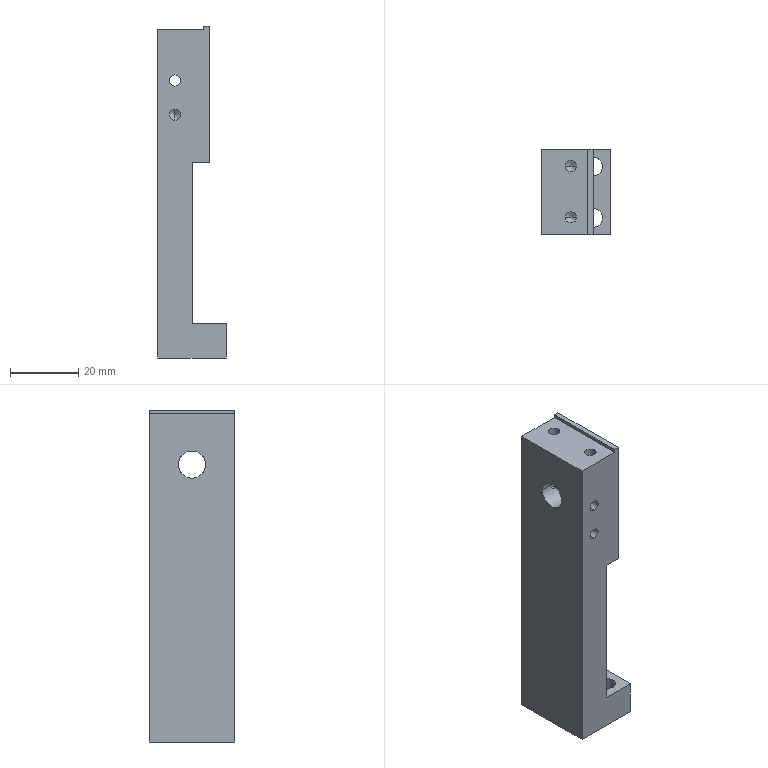Part | STEP file | 11-FG-B02911 | 1 solid | 38 faces | box 20 x 25 x 97.4 mm | volume 29767 mm3 | cylinder 18 | plane 12 | cone 8 | commonest cylinder face diameters 3.3 x12 5.5 x4 8 x2
STEP:
#1=CARTESIAN_POINT('',(5.,14.9,69.75));
#2=VERTEX_POINT('',#1);
#3=CARTESIAN_POINT('',(5.,14.9,73.05));
#4=VERTEX_POINT('',#3);
#5=CARTESIAN_POINT('',(5.,14.9,71.4));
#6=DIRECTION('',(0.,1.,0.));
#7=DIRECTION('',(0.,0.,1.));
#8=AXIS2_PLACEMENT_3D('',#5,#6,#7);
#9=CIRCLE('',#8,1.65);
#10=EDGE_CURVE('',#2,#4,#9,.T.);
#11=ORIENTED_EDGE('',*,*,#10,.F.);
#12=CARTESIAN_POINT('',(5.,25.,69.75));
#13=VERTEX_POINT('',#12);
#14=CARTESIAN_POINT('',(5.,25.,69.75));
#15=DIRECTION('',(0.,1.,0.));
#16=VECTOR('',#15,1000.);
#17=LINE('',#14,#16);
#18=EDGE_CURVE('',#2,#13,#17,.T.);
#19=ORIENTED_EDGE('',*,*,#18,.T.);
#20=CARTESIAN_POINT('',(5.,25.,73.05));
#21=VERTEX_POINT('',#20);
#22=CARTESIAN_POINT('',(5.,25.,71.4));
#23=DIRECTION('',(0.,1.,0.));
#24=DIRECTION('',(0.,0.,1.));
#25=AXIS2_PLACEMENT_3D('',#22,#23,#24);
#26=CIRCLE('',#25,1.65);
#27=EDGE_CURVE('',#13,#21,#26,.T.);
#28=ORIENTED_EDGE('',*,*,#27,.T.);
#29=CARTESIAN_POINT('',(5.,25.,73.05));
#30=DIRECTION('',(0.,1.,0.));
#31=VECTOR('',#30,1000.);
#32=LINE('',#29,#31);
#33=EDGE_CURVE('',#4,#21,#32,.T.);
#34=ORIENTED_EDGE('',*,*,#33,.F.);
#35=EDGE_LOOP('',(#11,#19,#28,#34));
#36=FACE_OUTER_BOUND('',#35,.T.);
#37=CARTESIAN_POINT('',(5.,25.,71.4));
#38=DIRECTION('',(0.,1.,0.));
#39=DIRECTION('',(0.,0.,1.));
#40=AXIS2_PLACEMENT_3D('',#37,#38,#39);
#41=CYLINDRICAL_SURFACE('',#40,1.65);
#42=ADVANCED_FACE('',(#36),#41,.F.);
#43=CARTESIAN_POINT('',(5.,13.909,71.4));
#44=VERTEX_POINT('',#43);
#45=CARTESIAN_POINT('',(5.,14.9,73.05));
#46=DIRECTION('',(0.,0.515,0.8572));
#47=VECTOR('',#46,1000.);
#48=LINE('',#45,#47);
#49=EDGE_CURVE('',#44,#4,#48,.T.);
#50=ORIENTED_EDGE('',*,*,#49,.F.);
#51=CARTESIAN_POINT('',(5.,14.9,69.75));
#52=DIRECTION('',(0.,0.515,-0.8572));
#53=VECTOR('',#52,1000.);
#54=LINE('',#51,#53);
#55=EDGE_CURVE('',#44,#2,#54,.T.);
#56=ORIENTED_EDGE('',*,*,#55,.T.);
#57=ORIENTED_EDGE('',*,*,#10,.T.);
#58=EDGE_LOOP('',(#50,#56,#57));
#59=FACE_OUTER_BOUND('',#58,.T.);
#60=CARTESIAN_POINT('',(5.,14.9,71.4));
#61=DIRECTION('',(0.,1.,0.));
#62=DIRECTION('',(0.,0.,1.));
#63=AXIS2_PLACEMENT_3D('',#60,#61,#62);
#64=CONICAL_SURFACE('',#63,1.65,1.03);
#65=ADVANCED_FACE('',(#59),#64,.F.);
#66=CARTESIAN_POINT('',(5.,10.1,73.05));
#67=VERTEX_POINT('',#66);
#68=CARTESIAN_POINT('',(5.,10.1,69.75));
#69=VERTEX_POINT('',#68);
#70=CARTESIAN_POINT('',(5.,10.1,71.4));
#71=DIRECTION('',(0.,-1.,0.));
#72=DIRECTION('',(0.,0.,-1.));
#73=AXIS2_PLACEMENT_3D('',#70,#71,#72);
#74=CIRCLE('',#73,1.65);
#75=EDGE_CURVE('',#67,#69,#74,.T.);
#76=ORIENTED_EDGE('',*,*,#75,.F.);
#77=CARTESIAN_POINT('',(5.,0.,73.05));
#78=VERTEX_POINT('',#77);
#79=CARTESIAN_POINT('',(5.,0.,73.05));
#80=DIRECTION('',(0.,-1.,0.));
#81=VECTOR('',#80,1000.);
#82=LINE('',#79,#81);
#83=EDGE_CURVE('',#67,#78,#82,.T.);
#84=ORIENTED_EDGE('',*,*,#83,.T.);
#85=CARTESIAN_POINT('',(5.,0.,69.75));
#86=VERTEX_POINT('',#85);
#87=CARTESIAN_POINT('',(5.,0.,71.4));
#88=DIRECTION('',(0.,-1.,0.));
#89=DIRECTION('',(0.,0.,-1.));
#90=AXIS2_PLACEMENT_3D('',#87,#88,#89);
#91=CIRCLE('',#90,1.65);
#92=EDGE_CURVE('',#78,#86,#91,.T.);
#93=ORIENTED_EDGE('',*,*,#92,.T.);
#94=CARTESIAN_POINT('',(5.,0.,69.75));
#95=DIRECTION('',(0.,-1.,0.));
#96=VECTOR('',#95,1000.);
#97=LINE('',#94,#96);
#98=EDGE_CURVE('',#69,#86,#97,.T.);
#99=ORIENTED_EDGE('',*,*,#98,.F.);
#100=EDGE_LOOP('',(#76,#84,#93,#99));
#101=FACE_OUTER_BOUND('',#100,.T.);
#102=CARTESIAN_POINT('',(5.,0.,71.4));
#103=DIRECTION('',(0.,-1.,0.));
#104=DIRECTION('',(0.,0.,-1.));
#105=AXIS2_PLACEMENT_3D('',#102,#103,#104);
#106=CYLINDRICAL_SURFACE('',#105,1.65);
#107=ADVANCED_FACE('',(#101),#106,.F.);
#108=CARTESIAN_POINT('',(5.,11.091,71.4));
#109=VERTEX_POINT('',#108);
#110=CARTESIAN_POINT('',(5.,10.1,69.75));
#111=DIRECTION('',(0.,-0.515,-0.8572));
#112=VECTOR('',#111,1000.);
#113=LINE('',#110,#112);
#114=EDGE_CURVE('',#109,#69,#113,.T.);
#115=ORIENTED_EDGE('',*,*,#114,.F.);
#116=CARTESIAN_POINT('',(5.,10.1,73.05));
#117=DIRECTION('',(0.,-0.515,0.8572));
#118=VECTOR('',#117,1000.);
#119=LINE('',#116,#118);
#120=EDGE_CURVE('',#109,#67,#119,.T.);
#121=ORIENTED_EDGE('',*,*,#120,.T.);
#122=ORIENTED_EDGE('',*,*,#75,.T.);
#123=EDGE_LOOP('',(#115,#121,#122));
#124=FACE_OUTER_BOUND('',#123,.T.);
#125=CARTESIAN_POINT('',(5.,10.1,71.4));
#126=DIRECTION('',(0.,-1.,0.));
#127=DIRECTION('',(0.,0.,-1.));
#128=AXIS2_PLACEMENT_3D('',#125,#126,#127);
#129=CONICAL_SURFACE('',#128,1.65,1.03);
#130=ADVANCED_FACE('',(#124),#129,.F.);
#131=CARTESIAN_POINT('',(5.,16.144,79.75));
#132=VERTEX_POINT('',#131);
#133=CARTESIAN_POINT('',(3.35,16.5,81.4));
#134=VERTEX_POINT('',#133);
#135=CARTESIAN_POINT('',(5.,16.144,79.75));
#136=CARTESIAN_POINT('',(4.891,16.144,79.75));
#137=CARTESIAN_POINT('',(4.781,16.149,79.761));
#138=CARTESIAN_POINT('',(4.568,16.168,79.804));
#139=CARTESIAN_POINT('',(4.464,16.182,79.836));
#140=CARTESIAN_POINT('',(4.165,16.233,79.961));
#141=CARTESIAN_POINT('',(3.985,16.28,80.082));
#142=CARTESIAN_POINT('',(3.757,16.349,80.31));
#143=CARTESIAN_POINT('',(3.689,16.372,80.392));
#144=CARTESIAN_POINT('',(3.571,16.414,80.569));
#145=CARTESIAN_POINT('',(3.519,16.433,80.665));
#146=CARTESIAN_POINT('',(3.436,16.465,80.865));
#147=CARTESIAN_POINT('',(3.404,16.478,80.968));
#148=CARTESIAN_POINT('',(3.361,16.495,81.181));
#149=CARTESIAN_POINT('',(3.35,16.5,81.291));
#150=CARTESIAN_POINT('',(3.35,16.5,81.4));
#151=B_SPLINE_CURVE_WITH_KNOTS('',3,(#135,#136,#137,#138,#139,#140,#141,#142,#143,#144,#145,#146,#147,#148,#149,#150),.UNSPECIFIED.,.F.,.F.,(4,2,2,2,2,2,2,4),(0.005217,0.005543,0.005869,0.006521,0.006847,0.007172,0.007498,0.007824),.UNSPECIFIED.);
#152=EDGE_CURVE('',#132,#134,#151,.T.);
#153=ORIENTED_EDGE('',*,*,#152,.F.);
#154=CARTESIAN_POINT('',(5.,25.,79.75));
#155=VERTEX_POINT('',#154);
#156=CARTESIAN_POINT('',(5.,25.,79.75));
#157=DIRECTION('',(0.,1.,0.));
#158=VECTOR('',#157,1000.);
#159=LINE('',#156,#158);
#160=EDGE_CURVE('',#132,#155,#159,.T.);
#161=ORIENTED_EDGE('',*,*,#160,.T.);
#162=CARTESIAN_POINT('',(5.,25.,83.05));
#163=VERTEX_POINT('',#162);
#164=CARTESIAN_POINT('',(5.,25.,81.4));
#165=DIRECTION('',(0.,1.,0.));
#166=DIRECTION('',(0.,0.,1.));
#167=AXIS2_PLACEMENT_3D('',#164,#165,#166);
#168=CIRCLE('',#167,1.65);
#169=EDGE_CURVE('',#155,#163,#168,.T.);
#170=ORIENTED_EDGE('',*,*,#169,.T.);
#171=CARTESIAN_POINT('',(5.,16.144,83.05));
#172=VERTEX_POINT('',#171);
#173=CARTESIAN_POINT('',(5.,25.,83.05));
#174=DIRECTION('',(0.,1.,0.));
#175=VECTOR('',#174,1000.);
#176=LINE('',#173,#175);
#177=EDGE_CURVE('',#172,#163,#176,.T.);
#178=ORIENTED_EDGE('',*,*,#177,.F.);
#179=CARTESIAN_POINT('',(3.35,16.5,81.4));
#180=CARTESIAN_POINT('',(3.35,16.5,81.618));
#181=CARTESIAN_POINT('',(3.394,16.481,81.837));
#182=CARTESIAN_POINT('',(3.519,16.433,82.135));
#183=CARTESIAN_POINT('',(3.571,16.414,82.231));
#184=CARTESIAN_POINT('',(3.69,16.372,82.409));
#185=CARTESIAN_POINT('',(3.758,16.349,82.491));
#186=CARTESIAN_POINT('',(3.909,16.303,82.643));
#187=CARTESIAN_POINT('',(3.993,16.279,82.711));
#188=CARTESIAN_POINT('',(4.17,16.236,82.83));
#189=CARTESIAN_POINT('',(4.264,16.216,82.881));
#190=CARTESIAN_POINT('',(4.565,16.164,83.007));
#191=CARTESIAN_POINT('',(4.779,16.144,83.05));
#192=CARTESIAN_POINT('',(5.,16.144,83.05));
#193=B_SPLINE_CURVE_WITH_KNOTS('',3,(#179,#180,#181,#182,#183,#184,#185,#186,#187,#188,#189,#190,#191,#192),.UNSPECIFIED.,.F.,.F.,(4,2,2,2,2,2,4),(0.007824,0.008476,0.008802,0.009127,0.009453,0.009779,0.01043),.UNSPECIFIED.);
#194=EDGE_CURVE('',#134,#172,#193,.T.);
#195=ORIENTED_EDGE('',*,*,#194,.F.);
#196=EDGE_LOOP('',(#153,#161,#170,#178,#195));
#197=FACE_OUTER_BOUND('',#196,.T.);
#198=CARTESIAN_POINT('',(5.,25.,81.4));
#199=DIRECTION('',(0.,1.,0.));
#200=DIRECTION('',(0.,0.,1.));
#201=AXIS2_PLACEMENT_3D('',#198,#199,#200);
#202=CYLINDRICAL_SURFACE('',#201,1.65);
#203=ADVANCED_FACE('',(#197),#202,.F.);
#204=CARTESIAN_POINT('',(12.25,5.,0.));
#205=VERTEX_POINT('',#204);
#206=CARTESIAN_POINT('',(17.75,5.,0.));
#207=VERTEX_POINT('',#206);
#208=CARTESIAN_POINT('',(15.,5.,0.));
#209=DIRECTION('',(0.,0.,1.));
#210=DIRECTION('',(1.,0.,0.));
#211=AXIS2_PLACEMENT_3D('',#208,#209,#210);
#212=CIRCLE('',#211,2.75);
#213=EDGE_CURVE('',#205,#207,#212,.T.);
#214=ORIENTED_EDGE('',*,*,#213,.F.);
#215=CARTESIAN_POINT('',(12.25,5.,10.));
#216=VERTEX_POINT('',#215);
#217=CARTESIAN_POINT('',(12.25,5.,0.));
#218=DIRECTION('',(0.,0.,1.));
#219=VECTOR('',#218,1000.);
#220=LINE('',#217,#219);
#221=EDGE_CURVE('',#205,#216,#220,.T.);
#222=ORIENTED_EDGE('',*,*,#221,.T.);
#223=CARTESIAN_POINT('',(17.75,5.,10.));
#224=VERTEX_POINT('',#223);
#225=CARTESIAN_POINT('',(15.,5.,10.));
#226=DIRECTION('',(0.,0.,1.));
#227=DIRECTION('',(1.,0.,0.));
#228=AXIS2_PLACEMENT_3D('',#225,#226,#227);
#229=CIRCLE('',#228,2.75);
#230=EDGE_CURVE('',#216,#224,#229,.T.);
#231=ORIENTED_EDGE('',*,*,#230,.T.);
#232=CARTESIAN_POINT('',(17.75,5.,0.));
#233=DIRECTION('',(0.,0.,1.));
#234=VECTOR('',#233,1000.);
#235=LINE('',#232,#234);
#236=EDGE_CURVE('',#207,#224,#235,.T.);
#237=ORIENTED_EDGE('',*,*,#236,.F.);
#238=EDGE_LOOP('',(#214,#222,#231,#237));
#239=FACE_OUTER_BOUND('',#238,.T.);
#240=CARTESIAN_POINT('',(15.,5.,0.));
#241=DIRECTION('',(0.,0.,1.));
#242=DIRECTION('',(1.,0.,0.));
#243=AXIS2_PLACEMENT_3D('',#240,#241,#242);
#244=CYLINDRICAL_SURFACE('',#243,2.75);
#245=ADVANCED_FACE('',(#239),#244,.F.);
#246=CARTESIAN_POINT('',(12.25,20.,0.));
#247=VERTEX_POINT('',#246);
#248=CARTESIAN_POINT('',(17.75,20.,0.));
#249=VERTEX_POINT('',#248);
#250=CARTESIAN_POINT('',(15.,20.,0.));
#251=DIRECTION('',(0.,0.,1.));
#252=DIRECTION('',(1.,0.,0.));
#253=AXIS2_PLACEMENT_3D('',#250,#251,#252);
#254=CIRCLE('',#253,2.75);
#255=EDGE_CURVE('',#247,#249,#254,.T.);
#256=ORIENTED_EDGE('',*,*,#255,.F.);
#257=CARTESIAN_POINT('',(12.25,20.,10.));
#258=VERTEX_POINT('',#257);
#259=CARTESIAN_POINT('',(12.25,20.,0.));
#260=DIRECTION('',(0.,0.,1.));
#261=VECTOR('',#260,1000.);
#262=LINE('',#259,#261);
#263=EDGE_CURVE('',#247,#258,#262,.T.);
#264=ORIENTED_EDGE('',*,*,#263,.T.);
#265=CARTESIAN_POINT('',(17.75,20.,10.));
#266=VERTEX_POINT('',#265);
#267=CARTESIAN_POINT('',(15.,20.,10.));
#268=DIRECTION('',(0.,0.,1.));
#269=DIRECTION('',(1.,0.,0.));
#270=AXIS2_PLACEMENT_3D('',#267,#268,#269);
#271=CIRCLE('',#270,2.75);
#272=EDGE_CURVE('',#258,#266,#271,.T.);
#273=ORIENTED_EDGE('',*,*,#272,.T.);
#274=CARTESIAN_POINT('',(17.75,20.,0.));
#275=DIRECTION('',(0.,0.,1.));
#276=VECTOR('',#275,1000.);
#277=LINE('',#274,#276);
#278=EDGE_CURVE('',#249,#266,#277,.T.);
#279=ORIENTED_EDGE('',*,*,#278,.F.);
#280=EDGE_LOOP('',(#256,#264,#273,#279));
#281=FACE_OUTER_BOUND('',#280,.T.);
#282=CARTESIAN_POINT('',(15.,20.,0.));
#283=DIRECTION('',(0.,0.,1.));
#284=DIRECTION('',(1.,0.,0.));
#285=AXIS2_PLACEMENT_3D('',#282,#283,#284);
#286=CYLINDRICAL_SURFACE('',#285,2.75);
#287=ADVANCED_FACE('',(#281),#286,.F.);
#288=CARTESIAN_POINT('',(5.,8.856,83.05));
#289=VERTEX_POINT('',#288);
#290=CARTESIAN_POINT('',(3.35,8.5,81.4));
#291=VERTEX_POINT('',#290);
#292=CARTESIAN_POINT('',(5.,8.856,83.05));
#293=CARTESIAN_POINT('',(4.891,8.856,83.05));
#294=CARTESIAN_POINT('',(4.78,8.851,83.039));
#295=CARTESIAN_POINT('',(4.568,8.832,82.996));
#296=CARTESIAN_POINT('',(4.464,8.818,82.964));
#297=CARTESIAN_POINT('',(4.263,8.784,82.88));
#298=CARTESIAN_POINT('',(4.169,8.764,82.829));
#299=CARTESIAN_POINT('',(3.992,8.72,82.71));
#300=CARTESIAN_POINT('',(3.908,8.697,82.641));
#301=CARTESIAN_POINT('',(3.757,8.651,82.491));
#302=CARTESIAN_POINT('',(3.69,8.628,82.408));
#303=CARTESIAN_POINT('',(3.57,8.586,82.23));
#304=CARTESIAN_POINT('',(3.518,8.567,82.134));
#305=CARTESIAN_POINT('',(3.394,8.519,81.837));
#306=CARTESIAN_POINT('',(3.35,8.5,81.617));
#307=CARTESIAN_POINT('',(3.35,8.5,81.4));
#308=B_SPLINE_CURVE_WITH_KNOTS('',3,(#292,#293,#294,#295,#296,#297,#298,#299,#300,#301,#302,#303,#304,#305,#306,#307),.UNSPECIFIED.,.F.,.F.,(4,2,2,2,2,2,2,4),(0.00261,0.002936,0.003262,0.003588,0.003914,0.00424,0.004566,0.005218),.UNSPECIFIED.);
#309=EDGE_CURVE('',#289,#291,#308,.T.);
#310=ORIENTED_EDGE('',*,*,#309,.F.);
#311=CARTESIAN_POINT('',(5.,0.,83.05));
#312=VERTEX_POINT('',#311);
#313=CARTESIAN_POINT('',(5.,0.,83.05));
#314=DIRECTION('',(0.,-1.,0.));
#315=VECTOR('',#314,1000.);
#316=LINE('',#313,#315);
#317=EDGE_CURVE('',#289,#312,#316,.T.);
#318=ORIENTED_EDGE('',*,*,#317,.T.);
#319=CARTESIAN_POINT('',(5.,0.,79.75));
#320=VERTEX_POINT('',#319);
#321=CARTESIAN_POINT('',(5.,0.,81.4));
#322=DIRECTION('',(0.,-1.,0.));
#323=DIRECTION('',(0.,0.,-1.));
#324=AXIS2_PLACEMENT_3D('',#321,#322,#323);
#325=CIRCLE('',#324,1.65);
#326=EDGE_CURVE('',#312,#320,#325,.T.);
#327=ORIENTED_EDGE('',*,*,#326,.T.);
#328=CARTESIAN_POINT('',(5.,8.856,79.75));
#329=VERTEX_POINT('',#328);
#330=CARTESIAN_POINT('',(5.,0.,79.75));
#331=DIRECTION('',(0.,-1.,0.));
#332=VECTOR('',#331,1000.);
#333=LINE('',#330,#332);
#334=EDGE_CURVE('',#329,#320,#333,.T.);
#335=ORIENTED_EDGE('',*,*,#334,.F.);
#336=CARTESIAN_POINT('',(3.35,8.5,81.4));
#337=CARTESIAN_POINT('',(3.35,8.5,81.291));
#338=CARTESIAN_POINT('',(3.361,8.505,81.181));
#339=CARTESIAN_POINT('',(3.404,8.522,80.967));
#340=CARTESIAN_POINT('',(3.436,8.535,80.864));
#341=CARTESIAN_POINT('',(3.561,8.583,80.564));
#342=CARTESIAN_POINT('',(3.682,8.628,80.384));
#343=CARTESIAN_POINT('',(3.91,8.697,80.156));
#344=CARTESIAN_POINT('',(3.993,8.72,80.089));
#345=CARTESIAN_POINT('',(4.17,8.764,79.97));
#346=CARTESIAN_POINT('',(4.266,8.784,79.918));
#347=CARTESIAN_POINT('',(4.465,8.818,79.835));
#348=CARTESIAN_POINT('',(4.568,8.832,79.804));
#349=CARTESIAN_POINT('',(4.781,8.851,79.761));
#350=CARTESIAN_POINT('',(4.891,8.856,79.75));
#351=CARTESIAN_POINT('',(5.,8.856,79.75));
#352=B_SPLINE_CURVE_WITH_KNOTS('',3,(#336,#337,#338,#339,#340,#341,#342,#343,#344,#345,#346,#347,#348,#349,#350,#351),.UNSPECIFIED.,.F.,.F.,(4,2,2,2,2,2,2,4),(0.005218,0.005543,0.005869,0.006521,0.006847,0.007173,0.007499,0.007825),.UNSPECIFIED.);
#353=EDGE_CURVE('',#291,#329,#352,.T.);
#354=ORIENTED_EDGE('',*,*,#353,.F.);
#355=EDGE_LOOP('',(#310,#318,#327,#335,#354));
#356=FACE_OUTER_BOUND('',#355,.T.);
#357=CARTESIAN_POINT('',(5.,0.,81.4));
#358=DIRECTION('',(0.,-1.,0.));
#359=DIRECTION('',(0.,0.,-1.));
#360=AXIS2_PLACEMENT_3D('',#357,#358,#359);
#361=CYLINDRICAL_SURFACE('',#360,1.65);
#362=ADVANCED_FACE('',(#356),#361,.F.);
#363=CARTESIAN_POINT('',(6.85,5.,86.3));
#364=VERTEX_POINT('',#363);
#365=CARTESIAN_POINT('',(10.15,5.,86.3));
#366=VERTEX_POINT('',#365);
#367=CARTESIAN_POINT('',(8.5,5.,86.3));
#368=DIRECTION('',(0.,0.,1.));
#369=DIRECTION('',(1.,0.,0.));
#370=AXIS2_PLACEMENT_3D('',#367,#368,#369);
#371=CIRCLE('',#370,1.65);
#372=EDGE_CURVE('',#364,#366,#371,.T.);
#373=ORIENTED_EDGE('',*,*,#372,.F.);
#374=CARTESIAN_POINT('',(6.85,5.,96.4));
#375=VERTEX_POINT('',#374);
#376=CARTESIAN_POINT('',(6.85,5.,96.4));
#377=DIRECTION('',(0.,0.,1.));
#378=VECTOR('',#377,1000.);
#379=LINE('',#376,#378);
#380=EDGE_CURVE('',#364,#375,#379,.T.);
#381=ORIENTED_EDGE('',*,*,#380,.T.);
#382=CARTESIAN_POINT('',(10.15,5.,96.4));
#383=VERTEX_POINT('',#382);
#384=CARTESIAN_POINT('',(8.5,5.,96.4));
#385=DIRECTION('',(0.,0.,1.));
#386=DIRECTION('',(1.,0.,0.));
#387=AXIS2_PLACEMENT_3D('',#384,#385,#386);
#388=CIRCLE('',#387,1.65);
#389=EDGE_CURVE('',#375,#383,#388,.T.);
#390=ORIENTED_EDGE('',*,*,#389,.T.);
#391=CARTESIAN_POINT('',(10.15,5.,96.4));
#392=DIRECTION('',(0.,0.,1.));
#393=VECTOR('',#392,1000.);
#394=LINE('',#391,#393);
#395=EDGE_CURVE('',#366,#383,#394,.T.);
#396=ORIENTED_EDGE('',*,*,#395,.F.);
#397=EDGE_LOOP('',(#373,#381,#390,#396));
#398=FACE_OUTER_BOUND('',#397,.T.);
#399=CARTESIAN_POINT('',(8.5,5.,96.4));
#400=DIRECTION('',(0.,0.,1.));
#401=DIRECTION('',(1.,0.,0.));
#402=AXIS2_PLACEMENT_3D('',#399,#400,#401);
#403=CYLINDRICAL_SURFACE('',#402,1.65);
#404=ADVANCED_FACE('',(#398),#403,.F.);
#405=CARTESIAN_POINT('',(8.5,5.,85.309));
#406=VERTEX_POINT('',#405);
#407=CARTESIAN_POINT('',(10.15,5.,86.3));
#408=DIRECTION('',(0.8572,0.,0.515));
#409=VECTOR('',#408,1000.);
#410=LINE('',#407,#409);
#411=EDGE_CURVE('',#406,#366,#410,.T.);
#412=ORIENTED_EDGE('',*,*,#411,.F.);
#413=CARTESIAN_POINT('',(6.85,5.,86.3));
#414=DIRECTION('',(-0.8572,0.,0.515));
#415=VECTOR('',#414,1000.);
#416=LINE('',#413,#415);
#417=EDGE_CURVE('',#406,#364,#416,.T.);
#418=ORIENTED_EDGE('',*,*,#417,.T.);
#419=ORIENTED_EDGE('',*,*,#372,.T.);
#420=EDGE_LOOP('',(#412,#418,#419));
#421=FACE_OUTER_BOUND('',#420,.T.);
#422=CARTESIAN_POINT('',(8.5,5.,86.3));
#423=DIRECTION('',(0.,0.,1.));
#424=DIRECTION('',(1.,0.,0.));
#425=AXIS2_PLACEMENT_3D('',#422,#423,#424);
#426=CONICAL_SURFACE('',#425,1.65,1.03);
#427=ADVANCED_FACE('',(#421),#426,.F.);
#428=CARTESIAN_POINT('',(6.85,20.,86.3));
#429=VERTEX_POINT('',#428);
#430=CARTESIAN_POINT('',(10.15,20.,86.3));
#431=VERTEX_POINT('',#430);
#432=CARTESIAN_POINT('',(8.5,20.,86.3));
#433=DIRECTION('',(0.,0.,1.));
#434=DIRECTION('',(1.,0.,0.));
#435=AXIS2_PLACEMENT_3D('',#432,#433,#434);
#436=CIRCLE('',#435,1.65);
#437=EDGE_CURVE('',#429,#431,#436,.T.);
#438=ORIENTED_EDGE('',*,*,#437,.F.);
#439=CARTESIAN_POINT('',(6.85,20.,96.4));
#440=VERTEX_POINT('',#439);
#441=CARTESIAN_POINT('',(6.85,20.,96.4));
#442=DIRECTION('',(0.,0.,1.));
#443=VECTOR('',#442,1000.);
#444=LINE('',#441,#443);
#445=EDGE_CURVE('',#429,#440,#444,.T.);
#446=ORIENTED_EDGE('',*,*,#445,.T.);
#447=CARTESIAN_POINT('',(10.15,20.,96.4));
#448=VERTEX_POINT('',#447);
#449=CARTESIAN_POINT('',(8.5,20.,96.4));
#450=DIRECTION('',(0.,0.,1.));
#451=DIRECTION('',(1.,0.,0.));
#452=AXIS2_PLACEMENT_3D('',#449,#450,#451);
#453=CIRCLE('',#452,1.65);
#454=EDGE_CURVE('',#440,#448,#453,.T.);
#455=ORIENTED_EDGE('',*,*,#454,.T.);
#456=CARTESIAN_POINT('',(10.15,20.,96.4));
#457=DIRECTION('',(0.,0.,1.));
#458=VECTOR('',#457,1000.);
#459=LINE('',#456,#458);
#460=EDGE_CURVE('',#431,#448,#459,.T.);
#461=ORIENTED_EDGE('',*,*,#460,.F.);
#462=EDGE_LOOP('',(#438,#446,#455,#461));
#463=FACE_OUTER_BOUND('',#462,.T.);
#464=CARTESIAN_POINT('',(8.5,20.,96.4));
#465=DIRECTION('',(0.,0.,1.));
#466=DIRECTION('',(1.,0.,0.));
#467=AXIS2_PLACEMENT_3D('',#464,#465,#466);
#468=CYLINDRICAL_SURFACE('',#467,1.65);
#469=ADVANCED_FACE('',(#463),#468,.F.);
#470=CARTESIAN_POINT('',(8.5,20.,85.309));
#471=VERTEX_POINT('',#470);
#472=CARTESIAN_POINT('',(10.15,20.,86.3));
#473=DIRECTION('',(0.8572,0.,0.515));
#474=VECTOR('',#473,1000.);
#475=LINE('',#472,#474);
#476=EDGE_CURVE('',#471,#431,#475,.T.);
#477=ORIENTED_EDGE('',*,*,#476,.F.);
#478=CARTESIAN_POINT('',(6.85,20.,86.3));
#479=DIRECTION('',(-0.8572,0.,0.515));
#480=VECTOR('',#479,1000.);
#481=LINE('',#478,#480);
#482=EDGE_CURVE('',#471,#429,#481,.T.);
#483=ORIENTED_EDGE('',*,*,#482,.T.);
#484=ORIENTED_EDGE('',*,*,#437,.T.);
#485=EDGE_LOOP('',(#477,#483,#484));
#486=FACE_OUTER_BOUND('',#485,.T.);
#487=CARTESIAN_POINT('',(8.5,20.,86.3));
#488=DIRECTION('',(0.,0.,1.));
#489=DIRECTION('',(1.,0.,0.));
#490=AXIS2_PLACEMENT_3D('',#487,#488,#489);
#491=CONICAL_SURFACE('',#490,1.65,1.03);
#492=ADVANCED_FACE('',(#486),#491,.F.);
#493=CARTESIAN_POINT('',(15.,16.5,81.4));
#494=VERTEX_POINT('',#493);
#495=CARTESIAN_POINT('',(15.,8.5,81.4));
#496=VERTEX_POINT('',#495);
#497=CARTESIAN_POINT('',(15.,12.5,81.4));
#498=DIRECTION('',(-1.,0.,0.));
#499=DIRECTION('',(0.,-1.,0.));
#500=AXIS2_PLACEMENT_3D('',#497,#498,#499);
#501=CIRCLE('',#500,4.);
#502=EDGE_CURVE('',#494,#496,#501,.T.);
#503=ORIENTED_EDGE('',*,*,#502,.F.);
#504=CARTESIAN_POINT('',(6.65,16.5,81.4));
#505=VERTEX_POINT('',#504);
#506=CARTESIAN_POINT('',(20.,16.5,81.4));
#507=DIRECTION('',(-1.,0.,0.));
#508=VECTOR('',#507,1000.);
#509=LINE('',#506,#508);
#510=EDGE_CURVE('',#494,#505,#509,.T.);
#511=ORIENTED_EDGE('',*,*,#510,.T.);
#512=CARTESIAN_POINT('',(6.65,16.5,81.4));
#513=CARTESIAN_POINT('',(6.65,16.5,81.291));
#514=CARTESIAN_POINT('',(6.639,16.495,81.18));
#515=CARTESIAN_POINT('',(6.596,16.478,80.968));
#516=CARTESIAN_POINT('',(6.564,16.465,80.864));
#517=CARTESIAN_POINT('',(6.48,16.433,80.663));
#518=CARTESIAN_POINT('',(6.429,16.414,80.568));
#519=CARTESIAN_POINT('',(6.31,16.372,80.391));
#520=CARTESIAN_POINT('',(6.241,16.349,80.307));
#521=CARTESIAN_POINT('',(6.09,16.303,80.156));
#522=CARTESIAN_POINT('',(6.008,16.28,80.089));
#523=CARTESIAN_POINT('',(5.829,16.236,79.97));
#524=CARTESIAN_POINT('',(5.734,16.216,79.918));
#525=CARTESIAN_POINT('',(5.437,16.165,79.794));
#526=CARTESIAN_POINT('',(5.217,16.144,79.75));
#527=CARTESIAN_POINT('',(5.,16.144,79.75));
#528=B_SPLINE_CURVE_WITH_KNOTS('',3,(#512,#513,#514,#515,#516,#517,#518,#519,#520,#521,#522,#523,#524,#525,#526,#527),.UNSPECIFIED.,.F.,.F.,(4,2,2,2,2,2,2,4),(0.00261,0.002935,0.003261,0.003587,0.003913,0.004239,0.004565,0.005217),.UNSPECIFIED.);
#529=EDGE_CURVE('',#505,#132,#528,.T.);
#530=ORIENTED_EDGE('',*,*,#529,.T.);
#531=ORIENTED_EDGE('',*,*,#152,.T.);
#532=CARTESIAN_POINT('',(0.,16.5,81.4));
#533=VERTEX_POINT('',#532);
#534=CARTESIAN_POINT('',(20.,16.5,81.4));
#535=DIRECTION('',(-1.,0.,0.));
#536=VECTOR('',#535,1000.);
#537=LINE('',#534,#536);
#538=EDGE_CURVE('',#134,#533,#537,.T.);
#539=ORIENTED_EDGE('',*,*,#538,.T.);
#540=CARTESIAN_POINT('',(0.,8.5,81.4));
#541=VERTEX_POINT('',#540);
#542=CARTESIAN_POINT('',(0.,12.5,81.4));
#543=DIRECTION('',(-1.,0.,0.));
#544=DIRECTION('',(0.,-1.,0.));
#545=AXIS2_PLACEMENT_3D('',#542,#543,#544);
#546=CIRCLE('',#545,4.);
#547=EDGE_CURVE('',#533,#541,#546,.T.);
#548=ORIENTED_EDGE('',*,*,#547,.T.);
#549=CARTESIAN_POINT('',(20.,8.5,81.4));
#550=DIRECTION('',(-1.,0.,0.));
#551=VECTOR('',#550,1000.);
#552=LINE('',#549,#551);
#553=EDGE_CURVE('',#291,#541,#552,.T.);
#554=ORIENTED_EDGE('',*,*,#553,.F.);
#555=ORIENTED_EDGE('',*,*,#353,.T.);
#556=CARTESIAN_POINT('',(6.65,8.5,81.4));
#557=VERTEX_POINT('',#556);
#558=CARTESIAN_POINT('',(5.,8.856,79.75));
#559=CARTESIAN_POINT('',(5.217,8.856,79.75));
#560=CARTESIAN_POINT('',(5.436,8.835,79.794));
#561=CARTESIAN_POINT('',(5.734,8.784,79.919));
#562=CARTESIAN_POINT('',(5.831,8.764,79.97));
#563=CARTESIAN_POINT('',(6.008,8.72,80.09));
#564=CARTESIAN_POINT('',(6.09,8.697,80.157));
#565=CARTESIAN_POINT('',(6.242,8.651,80.308));
#566=CARTESIAN_POINT('',(6.311,8.628,80.392));
#567=CARTESIAN_POINT('',(6.429,8.586,80.569));
#568=CARTESIAN_POINT('',(6.48,8.567,80.663));
#569=CARTESIAN_POINT('',(6.607,8.518,80.965));
#570=CARTESIAN_POINT('',(6.65,8.5,81.18));
#571=CARTESIAN_POINT('',(6.65,8.5,81.4));
#572=B_SPLINE_CURVE_WITH_KNOTS('',3,(#558,#559,#560,#561,#562,#563,#564,#565,#566,#567,#568,#569,#570,#571),.UNSPECIFIED.,.F.,.F.,(4,2,2,2,2,2,4),(0.007825,0.008476,0.008802,0.009128,0.009454,0.00978,0.01043),.UNSPECIFIED.);
#573=EDGE_CURVE('',#329,#557,#572,.T.);
#574=ORIENTED_EDGE('',*,*,#573,.T.);
#575=CARTESIAN_POINT('',(20.,8.5,81.4));
#576=DIRECTION('',(-1.,0.,0.));
#577=VECTOR('',#576,1000.);
#578=LINE('',#575,#577);
#579=EDGE_CURVE('',#496,#557,#578,.T.);
#580=ORIENTED_EDGE('',*,*,#579,.F.);
#581=EDGE_LOOP('',(#503,#511,#530,#531,#539,#548,#554,#555,#574,#580));
#582=FACE_OUTER_BOUND('',#581,.T.);
#583=CARTESIAN_POINT('',(20.,12.5,81.4));
#584=DIRECTION('',(-1.,0.,0.));
#585=DIRECTION('',(0.,-1.,0.));
#586=AXIS2_PLACEMENT_3D('',#583,#584,#585);
#587=CYLINDRICAL_SURFACE('',#586,4.);
#588=ADVANCED_FACE('',(#582),#587,.F.);
#589=CARTESIAN_POINT('',(8.5,20.,96.4));
#590=DIRECTION('',(0.,0.,1.));
#591=DIRECTION('',(1.,0.,0.));
#592=AXIS2_PLACEMENT_3D('',#589,#590,#591);
#593=CIRCLE('',#592,1.65);
#594=EDGE_CURVE('',#448,#440,#593,.T.);
#595=ORIENTED_EDGE('',*,*,#594,.F.);
#596=ORIENTED_EDGE('',*,*,#454,.F.);
#597=EDGE_LOOP('',(#595,#596));
#598=FACE_BOUND('',#597,.T.);
#599=CARTESIAN_POINT('',(8.5,5.,96.4));
#600=DIRECTION('',(0.,0.,1.));
#601=DIRECTION('',(1.,0.,0.));
#602=AXIS2_PLACEMENT_3D('',#599,#600,#601);
#603=CIRCLE('',#602,1.65);
#604=EDGE_CURVE('',#383,#375,#603,.T.);
#605=ORIENTED_EDGE('',*,*,#604,.F.);
#606=ORIENTED_EDGE('',*,*,#389,.F.);
#607=EDGE_LOOP('',(#605,#606));
#608=FACE_BOUND('',#607,.T.);
#609=CARTESIAN_POINT('',(13.5,25.,96.4));
#610=VERTEX_POINT('',#609);
#611=CARTESIAN_POINT('',(13.5,0.,96.4));
#612=VERTEX_POINT('',#611);
#613=CARTESIAN_POINT('',(13.5,25.,96.4));
#614=DIRECTION('',(0.,-1.,0.));
#615=VECTOR('',#614,1000.);
#616=LINE('',#613,#615);
#617=EDGE_CURVE('',#610,#612,#616,.T.);
#618=ORIENTED_EDGE('',*,*,#617,.F.);
#619=CARTESIAN_POINT('',(0.,25.,96.4));
#620=VERTEX_POINT('',#619);
#621=CARTESIAN_POINT('',(0.,25.,96.4));
#622=DIRECTION('',(-1.,0.,0.));
#623=VECTOR('',#622,1000.);
#624=LINE('',#621,#623);
#625=EDGE_CURVE('',#610,#620,#624,.T.);
#626=ORIENTED_EDGE('',*,*,#625,.T.);
#627=CARTESIAN_POINT('',(0.,0.,96.4));
#628=VERTEX_POINT('',#627);
#629=CARTESIAN_POINT('',(0.,0.,96.4));
#630=DIRECTION('',(0.,-1.,0.));
#631=VECTOR('',#630,1000.);
#632=LINE('',#629,#631);
#633=EDGE_CURVE('',#620,#628,#632,.T.);
#634=ORIENTED_EDGE('',*,*,#633,.T.);
#635=CARTESIAN_POINT('',(0.,0.,96.4));
#636=DIRECTION('',(1.,0.,0.));
#637=VECTOR('',#636,1000.);
#638=LINE('',#635,#637);
#639=EDGE_CURVE('',#628,#612,#638,.T.);
#640=ORIENTED_EDGE('',*,*,#639,.T.);
#641=EDGE_LOOP('',(#618,#626,#634,#640));
#642=FACE_OUTER_BOUND('',#641,.T.);
#643=CARTESIAN_POINT('',(0.,25.,96.4));
#644=DIRECTION('',(0.,0.,-1.));
#645=DIRECTION('',(-1.,0.,0.));
#646=AXIS2_PLACEMENT_3D('',#643,#644,#645);
#647=PLANE('',#646);
#648=ADVANCED_FACE('',(#598,#608,#642),#647,.F.);
#649=CARTESIAN_POINT('',(0.,12.5,81.4));
#650=DIRECTION('',(-1.,0.,0.));
#651=DIRECTION('',(0.,-1.,0.));
#652=AXIS2_PLACEMENT_3D('',#649,#650,#651);
#653=CIRCLE('',#652,4.);
#654=EDGE_CURVE('',#541,#533,#653,.T.);
#655=ORIENTED_EDGE('',*,*,#654,.F.);
#656=ORIENTED_EDGE('',*,*,#547,.F.);
#657=EDGE_LOOP('',(#655,#656));
#658=FACE_BOUND('',#657,.T.);
#659=CARTESIAN_POINT('',(0.,25.,0.));
#660=VERTEX_POINT('',#659);
#661=CARTESIAN_POINT('',(0.,0.,0.));
#662=VERTEX_POINT('',#661);
#663=CARTESIAN_POINT('',(0.,0.,0.));
#664=DIRECTION('',(0.,-1.,0.));
#665=VECTOR('',#664,1000.);
#666=LINE('',#663,#665);
#667=EDGE_CURVE('',#660,#662,#666,.T.);
#668=ORIENTED_EDGE('',*,*,#667,.T.);
#669=CARTESIAN_POINT('',(0.,0.,96.4));
#670=DIRECTION('',(0.,0.,-1.));
#671=VECTOR('',#670,1000.);
#672=LINE('',#669,#671);
#673=EDGE_CURVE('',#628,#662,#672,.T.);
#674=ORIENTED_EDGE('',*,*,#673,.F.);
#675=ORIENTED_EDGE('',*,*,#633,.F.);
#676=CARTESIAN_POINT('',(0.,25.,96.4));
#677=DIRECTION('',(0.,0.,-1.));
#678=VECTOR('',#677,1000.);
#679=LINE('',#676,#678);
#680=EDGE_CURVE('',#620,#660,#679,.T.);
#681=ORIENTED_EDGE('',*,*,#680,.T.);
#682=EDGE_LOOP('',(#668,#674,#675,#681));
#683=FACE_OUTER_BOUND('',#682,.T.);
#684=CARTESIAN_POINT('',(0.,0.,96.4));
#685=DIRECTION('',(1.,0.,0.));
#686=DIRECTION('',(0.,1.,0.));
#687=AXIS2_PLACEMENT_3D('',#684,#685,#686);
#688=PLANE('',#687);
#689=ADVANCED_FACE('',(#658,#683),#688,.F.);
#690=CARTESIAN_POINT('',(5.,0.,71.4));
#691=DIRECTION('',(0.,-1.,0.));
#692=DIRECTION('',(0.,0.,-1.));
#693=AXIS2_PLACEMENT_3D('',#690,#691,#692);
#694=CIRCLE('',#693,1.65);
#695=EDGE_CURVE('',#86,#78,#694,.T.);
#696=ORIENTED_EDGE('',*,*,#695,.F.);
#697=ORIENTED_EDGE('',*,*,#92,.F.);
#698=EDGE_LOOP('',(#696,#697));
#699=FACE_BOUND('',#698,.T.);
#700=CARTESIAN_POINT('',(5.,0.,81.4));
#701=DIRECTION('',(0.,-1.,0.));
#702=DIRECTION('',(0.,0.,-1.));
#703=AXIS2_PLACEMENT_3D('',#700,#701,#702);
#704=CIRCLE('',#703,1.65);
#705=EDGE_CURVE('',#320,#312,#704,.T.);
#706=ORIENTED_EDGE('',*,*,#705,.F.);
#707=ORIENTED_EDGE('',*,*,#326,.F.);
#708=EDGE_LOOP('',(#706,#707));
#709=FACE_BOUND('',#708,.T.);
#710=CARTESIAN_POINT('',(20.,0.,0.));
#711=VERTEX_POINT('',#710);
#712=CARTESIAN_POINT('',(0.,0.,0.));
#713=DIRECTION('',(1.,0.,0.));
#714=VECTOR('',#713,1000.);
#715=LINE('',#712,#714);
#716=EDGE_CURVE('',#662,#711,#715,.T.);
#717=ORIENTED_EDGE('',*,*,#716,.T.);
#718=CARTESIAN_POINT('',(20.,0.,10.));
#719=VERTEX_POINT('',#718);
#720=CARTESIAN_POINT('',(20.,0.,10.));
#721=DIRECTION('',(0.,0.,-1.));
#722=VECTOR('',#721,1000.);
#723=LINE('',#720,#722);
#724=EDGE_CURVE('',#719,#711,#723,.T.);
#725=ORIENTED_EDGE('',*,*,#724,.F.);
#726=CARTESIAN_POINT('',(10.,0.,10.));
#727=VERTEX_POINT('',#726);
#728=CARTESIAN_POINT('',(15.,0.,10.));
#729=DIRECTION('',(1.,0.,0.));
#730=VECTOR('',#729,1000.);
#731=LINE('',#728,#730);
#732=EDGE_CURVE('',#727,#719,#731,.T.);
#733=ORIENTED_EDGE('',*,*,#732,.F.);
#734=CARTESIAN_POINT('',(10.,0.,57.5));
#735=VERTEX_POINT('',#734);
#736=CARTESIAN_POINT('',(10.,0.,10.));
#737=DIRECTION('',(0.,0.,-1.));
#738=VECTOR('',#737,1000.);
#739=LINE('',#736,#738);
#740=EDGE_CURVE('',#735,#727,#739,.T.);
#741=ORIENTED_EDGE('',*,*,#740,.F.);
#742=CARTESIAN_POINT('',(15.,0.,57.5));
#743=VERTEX_POINT('',#742);
#744=CARTESIAN_POINT('',(15.,0.,57.5));
#745=DIRECTION('',(-1.,0.,0.));
#746=VECTOR('',#745,1000.);
#747=LINE('',#744,#746);
#748=EDGE_CURVE('',#743,#735,#747,.T.);
#749=ORIENTED_EDGE('',*,*,#748,.F.);
#750=CARTESIAN_POINT('',(15.,0.,97.4));
#751=VERTEX_POINT('',#750);
#752=CARTESIAN_POINT('',(15.,0.,96.4));
#753=DIRECTION('',(0.,0.,-1.));
#754=VECTOR('',#753,1000.);
#755=LINE('',#752,#754);
#756=EDGE_CURVE('',#751,#743,#755,.T.);
#757=ORIENTED_EDGE('',*,*,#756,.F.);
#758=CARTESIAN_POINT('',(13.5,0.,97.4));
#759=VERTEX_POINT('',#758);
#760=CARTESIAN_POINT('',(15.,0.,97.4));
#761=DIRECTION('',(1.,0.,0.));
#762=VECTOR('',#761,1000.);
#763=LINE('',#760,#762);
#764=EDGE_CURVE('',#759,#751,#763,.T.);
#765=ORIENTED_EDGE('',*,*,#764,.F.);
#766=CARTESIAN_POINT('',(13.5,0.,97.4));
#767=DIRECTION('',(0.,0.,-1.));
#768=VECTOR('',#767,1000.);
#769=LINE('',#766,#768);
#770=EDGE_CURVE('',#759,#612,#769,.T.);
#771=ORIENTED_EDGE('',*,*,#770,.T.);
#772=ORIENTED_EDGE('',*,*,#639,.F.);
#773=ORIENTED_EDGE('',*,*,#673,.T.);
#774=EDGE_LOOP('',(#717,#725,#733,#741,#749,#757,#765,#771,#772,#773));
#775=FACE_OUTER_BOUND('',#774,.T.);
#776=CARTESIAN_POINT('',(0.,0.,96.4));
#777=DIRECTION('',(0.,1.,0.));
#778=DIRECTION('',(0.,0.,1.));
#779=AXIS2_PLACEMENT_3D('',#776,#777,#778);
#780=PLANE('',#779);
#781=ADVANCED_FACE('',(#699,#709,#775),#780,.F.);
#782=CARTESIAN_POINT('',(15.,12.5,81.4));
#783=DIRECTION('',(-1.,0.,0.));
#784=DIRECTION('',(0.,-1.,0.));
#785=AXIS2_PLACEMENT_3D('',#782,#783,#784);
#786=CIRCLE('',#785,4.);
#787=EDGE_CURVE('',#496,#494,#786,.T.);
#788=ORIENTED_EDGE('',*,*,#787,.T.);
#789=ORIENTED_EDGE('',*,*,#502,.T.);
#790=EDGE_LOOP('',(#788,#789));
#791=FACE_BOUND('',#790,.T.);
#792=ORIENTED_EDGE('',*,*,#756,.T.);
#793=CARTESIAN_POINT('',(15.,25.,57.5));
#794=VERTEX_POINT('',#793);
#795=CARTESIAN_POINT('',(15.,72.,57.5));
#796=DIRECTION('',(0.,-1.,0.));
#797=VECTOR('',#796,1000.);
#798=LINE('',#795,#797);
#799=EDGE_CURVE('',#794,#743,#798,.T.);
#800=ORIENTED_EDGE('',*,*,#799,.F.);
#801=CARTESIAN_POINT('',(15.,25.,97.4));
#802=VERTEX_POINT('',#801);
#803=CARTESIAN_POINT('',(15.,25.,96.4));
#804=DIRECTION('',(0.,0.,-1.));
#805=VECTOR('',#804,1000.);
#806=LINE('',#803,#805);
#807=EDGE_CURVE('',#802,#794,#806,.T.);
#808=ORIENTED_EDGE('',*,*,#807,.F.);
#809=CARTESIAN_POINT('',(15.,25.,97.4));
#810=DIRECTION('',(0.,1.,0.));
#811=VECTOR('',#810,1000.);
#812=LINE('',#809,#811);
#813=EDGE_CURVE('',#751,#802,#812,.T.);
#814=ORIENTED_EDGE('',*,*,#813,.F.);
#815=EDGE_LOOP('',(#792,#800,#808,#814));
#816=FACE_OUTER_BOUND('',#815,.T.);
#817=CARTESIAN_POINT('',(15.,0.,96.4));
#818=DIRECTION('',(-1.,0.,0.));
#819=DIRECTION('',(0.,-1.,0.));
#820=AXIS2_PLACEMENT_3D('',#817,#818,#819);
#821=PLANE('',#820);
#822=ADVANCED_FACE('',(#791,#816),#821,.F.);
#823=CARTESIAN_POINT('',(5.,25.,71.4));
#824=DIRECTION('',(0.,1.,0.));
#825=DIRECTION('',(0.,0.,1.));
#826=AXIS2_PLACEMENT_3D('',#823,#824,#825);
#827=CIRCLE('',#826,1.65);
#828=EDGE_CURVE('',#21,#13,#827,.T.);
#829=ORIENTED_EDGE('',*,*,#828,.F.);
#830=ORIENTED_EDGE('',*,*,#27,.F.);
#831=EDGE_LOOP('',(#829,#830));
#832=FACE_BOUND('',#831,.T.);
#833=CARTESIAN_POINT('',(5.,25.,81.4));
#834=DIRECTION('',(0.,1.,0.));
#835=DIRECTION('',(0.,0.,1.));
#836=AXIS2_PLACEMENT_3D('',#833,#834,#835);
#837=CIRCLE('',#836,1.65);
#838=EDGE_CURVE('',#163,#155,#837,.T.);
#839=ORIENTED_EDGE('',*,*,#838,.F.);
#840=ORIENTED_EDGE('',*,*,#169,.F.);
#841=EDGE_LOOP('',(#839,#840));
#842=FACE_BOUND('',#841,.T.);
#843=CARTESIAN_POINT('',(10.,25.,57.5));
#844=VERTEX_POINT('',#843);
#845=CARTESIAN_POINT('',(10.,25.,10.));
#846=VERTEX_POINT('',#845);
#847=CARTESIAN_POINT('',(10.,25.,96.4));
#848=DIRECTION('',(0.,0.,-1.));
#849=VECTOR('',#848,1000.);
#850=LINE('',#847,#849);
#851=EDGE_CURVE('',#844,#846,#850,.T.);
#852=ORIENTED_EDGE('',*,*,#851,.T.);
#853=CARTESIAN_POINT('',(20.,25.,10.));
#854=VERTEX_POINT('',#853);
#855=CARTESIAN_POINT('',(0.,25.,10.));
#856=DIRECTION('',(1.,0.,0.));
#857=VECTOR('',#856,1000.);
#858=LINE('',#855,#857);
#859=EDGE_CURVE('',#846,#854,#858,.T.);
#860=ORIENTED_EDGE('',*,*,#859,.T.);
#861=CARTESIAN_POINT('',(20.,25.,0.));
#862=VERTEX_POINT('',#861);
#863=CARTESIAN_POINT('',(20.,25.,0.));
#864=DIRECTION('',(0.,0.,1.));
#865=VECTOR('',#864,1000.);
#866=LINE('',#863,#865);
#867=EDGE_CURVE('',#862,#854,#866,.T.);
#868=ORIENTED_EDGE('',*,*,#867,.F.);
#869=CARTESIAN_POINT('',(0.,25.,0.));
#870=DIRECTION('',(-1.,0.,0.));
#871=VECTOR('',#870,1000.);
#872=LINE('',#869,#871);
#873=EDGE_CURVE('',#862,#660,#872,.T.);
#874=ORIENTED_EDGE('',*,*,#873,.T.);
#875=ORIENTED_EDGE('',*,*,#680,.F.);
#876=ORIENTED_EDGE('',*,*,#625,.F.);
#877=CARTESIAN_POINT('',(13.5,25.,97.4));
#878=VERTEX_POINT('',#877);
#879=CARTESIAN_POINT('',(13.5,25.,97.4));
#880=DIRECTION('',(0.,0.,-1.));
#881=VECTOR('',#880,1000.);
#882=LINE('',#879,#881);
#883=EDGE_CURVE('',#878,#610,#882,.T.);
#884=ORIENTED_EDGE('',*,*,#883,.F.);
#885=CARTESIAN_POINT('',(15.,25.,97.4));
#886=DIRECTION('',(-1.,0.,0.));
#887=VECTOR('',#886,1000.);
#888=LINE('',#885,#887);
#889=EDGE_CURVE('',#802,#878,#888,.T.);
#890=ORIENTED_EDGE('',*,*,#889,.F.);
#891=ORIENTED_EDGE('',*,*,#807,.T.);
#892=CARTESIAN_POINT('',(0.,25.,57.5));
#893=DIRECTION('',(-1.,0.,0.));
#894=VECTOR('',#893,1000.);
#895=LINE('',#892,#894);
#896=EDGE_CURVE('',#794,#844,#895,.T.);
#897=ORIENTED_EDGE('',*,*,#896,.T.);
#898=EDGE_LOOP('',(#852,#860,#868,#874,#875,#876,#884,#890,#891,#897));
#899=FACE_OUTER_BOUND('',#898,.T.);
#900=CARTESIAN_POINT('',(0.,25.,96.4));
#901=DIRECTION('',(0.,-1.,0.));
#902=DIRECTION('',(0.,0.,-1.));
#903=AXIS2_PLACEMENT_3D('',#900,#901,#902);
#904=PLANE('',#903);
#905=ADVANCED_FACE('',(#832,#842,#899),#904,.F.);
#906=CARTESIAN_POINT('',(15.,5.,0.));
#907=DIRECTION('',(0.,0.,1.));
#908=DIRECTION('',(1.,0.,0.));
#909=AXIS2_PLACEMENT_3D('',#906,#907,#908);
#910=CIRCLE('',#909,2.75);
#911=EDGE_CURVE('',#207,#205,#910,.T.);
#912=ORIENTED_EDGE('',*,*,#911,.T.);
#913=ORIENTED_EDGE('',*,*,#213,.T.);
#914=EDGE_LOOP('',(#912,#913));
#915=FACE_BOUND('',#914,.T.);
#916=CARTESIAN_POINT('',(15.,20.,0.));
#917=DIRECTION('',(0.,0.,1.));
#918=DIRECTION('',(1.,0.,0.));
#919=AXIS2_PLACEMENT_3D('',#916,#917,#918);
#920=CIRCLE('',#919,2.75);
#921=EDGE_CURVE('',#249,#247,#920,.T.);
#922=ORIENTED_EDGE('',*,*,#921,.T.);
#923=ORIENTED_EDGE('',*,*,#255,.T.);
#924=EDGE_LOOP('',(#922,#923));
#925=FACE_BOUND('',#924,.T.);
#926=ORIENTED_EDGE('',*,*,#667,.F.);
#927=ORIENTED_EDGE('',*,*,#873,.F.);
#928=CARTESIAN_POINT('',(20.,0.,0.));
#929=DIRECTION('',(0.,1.,0.));
#930=VECTOR('',#929,1000.);
#931=LINE('',#928,#930);
#932=EDGE_CURVE('',#711,#862,#931,.T.);
#933=ORIENTED_EDGE('',*,*,#932,.F.);
#934=ORIENTED_EDGE('',*,*,#716,.F.);
#935=EDGE_LOOP('',(#926,#927,#933,#934));
#936=FACE_OUTER_BOUND('',#935,.T.);
#937=CARTESIAN_POINT('',(0.,25.,0.));
#938=DIRECTION('',(0.,0.,-1.));
#939=DIRECTION('',(-1.,0.,0.));
#940=AXIS2_PLACEMENT_3D('',#937,#938,#939);
#941=PLANE('',#940);
#942=ADVANCED_FACE('',(#915,#925,#936),#941,.T.);
#943=CARTESIAN_POINT('',(15.,5.,10.));
#944=DIRECTION('',(0.,0.,1.));
#945=DIRECTION('',(1.,0.,0.));
#946=AXIS2_PLACEMENT_3D('',#943,#944,#945);
#947=CIRCLE('',#946,2.75);
#948=EDGE_CURVE('',#224,#216,#947,.T.);
#949=ORIENTED_EDGE('',*,*,#948,.F.);
#950=ORIENTED_EDGE('',*,*,#230,.F.);
#951=EDGE_LOOP('',(#949,#950));
#952=FACE_BOUND('',#951,.T.);
#953=CARTESIAN_POINT('',(15.,20.,10.));
#954=DIRECTION('',(0.,0.,1.));
#955=DIRECTION('',(1.,0.,0.));
#956=AXIS2_PLACEMENT_3D('',#953,#954,#955);
#957=CIRCLE('',#956,2.75);
#958=EDGE_CURVE('',#266,#258,#957,.T.);
#959=ORIENTED_EDGE('',*,*,#958,.F.);
#960=ORIENTED_EDGE('',*,*,#272,.F.);
#961=EDGE_LOOP('',(#959,#960));
#962=FACE_BOUND('',#961,.T.);
#963=CARTESIAN_POINT('',(10.,72.,10.));
#964=DIRECTION('',(0.,-1.,0.));
#965=VECTOR('',#964,1000.);
#966=LINE('',#963,#965);
#967=EDGE_CURVE('',#846,#727,#966,.T.);
#968=ORIENTED_EDGE('',*,*,#967,.T.);
#969=ORIENTED_EDGE('',*,*,#732,.T.);
#970=CARTESIAN_POINT('',(20.,25.,10.));
#971=DIRECTION('',(0.,-1.,0.));
#972=VECTOR('',#971,1000.);
#973=LINE('',#970,#972);
#974=EDGE_CURVE('',#854,#719,#973,.T.);
#975=ORIENTED_EDGE('',*,*,#974,.F.);
#976=ORIENTED_EDGE('',*,*,#859,.F.);
#977=EDGE_LOOP('',(#968,#969,#975,#976));
#978=FACE_OUTER_BOUND('',#977,.T.);
#979=CARTESIAN_POINT('',(15.,72.,10.));
#980=DIRECTION('',(0.,0.,-1.));
#981=DIRECTION('',(-1.,0.,0.));
#982=AXIS2_PLACEMENT_3D('',#979,#980,#981);
#983=PLANE('',#982);
#984=ADVANCED_FACE('',(#952,#962,#978),#983,.F.);
#985=CARTESIAN_POINT('',(10.,72.,57.5));
#986=DIRECTION('',(0.,-1.,0.));
#987=VECTOR('',#986,1000.);
#988=LINE('',#985,#987);
#989=EDGE_CURVE('',#844,#735,#988,.T.);
#990=ORIENTED_EDGE('',*,*,#989,.T.);
#991=ORIENTED_EDGE('',*,*,#740,.T.);
#992=ORIENTED_EDGE('',*,*,#967,.F.);
#993=ORIENTED_EDGE('',*,*,#851,.F.);
#994=EDGE_LOOP('',(#990,#991,#992,#993));
#995=FACE_OUTER_BOUND('',#994,.T.);
#996=CARTESIAN_POINT('',(10.,72.,10.));
#997=DIRECTION('',(-1.,0.,0.));
#998=DIRECTION('',(0.,0.,1.));
#999=AXIS2_PLACEMENT_3D('',#996,#997,#998);
#1000=PLANE('',#999);
#1001=ADVANCED_FACE('',(#995),#1000,.F.);
#1002=ORIENTED_EDGE('',*,*,#799,.T.);
#1003=ORIENTED_EDGE('',*,*,#748,.T.);
#1004=ORIENTED_EDGE('',*,*,#989,.F.);
#1005=ORIENTED_EDGE('',*,*,#896,.F.);
#1006=EDGE_LOOP('',(#1002,#1003,#1004,#1005));
#1007=FACE_OUTER_BOUND('',#1006,.T.);
#1008=CARTESIAN_POINT('',(15.,72.,57.5));
#1009=DIRECTION('',(0.,0.,1.));
#1010=DIRECTION('',(1.,0.,0.));
#1011=AXIS2_PLACEMENT_3D('',#1008,#1009,#1010);
#1012=PLANE('',#1011);
#1013=ADVANCED_FACE('',(#1007),#1012,.F.);
#1014=ORIENTED_EDGE('',*,*,#932,.T.);
#1015=ORIENTED_EDGE('',*,*,#867,.T.);
#1016=ORIENTED_EDGE('',*,*,#974,.T.);
#1017=ORIENTED_EDGE('',*,*,#724,.T.);
#1018=EDGE_LOOP('',(#1014,#1015,#1016,#1017));
#1019=FACE_OUTER_BOUND('',#1018,.T.);
#1020=CARTESIAN_POINT('',(20.,25.,0.));
#1021=DIRECTION('',(1.,0.,0.));
#1022=DIRECTION('',(0.,1.,0.));
#1023=AXIS2_PLACEMENT_3D('',#1020,#1021,#1022);
#1024=PLANE('',#1023);
#1025=ADVANCED_FACE('',(#1019),#1024,.T.);
#1026=ORIENTED_EDGE('',*,*,#510,.F.);
#1027=ORIENTED_EDGE('',*,*,#787,.F.);
#1028=ORIENTED_EDGE('',*,*,#579,.T.);
#1029=CARTESIAN_POINT('',(6.65,8.5,81.4));
#1030=CARTESIAN_POINT('',(6.65,8.5,81.51));
#1031=CARTESIAN_POINT('',(6.639,8.505,81.619));
#1032=CARTESIAN_POINT('',(6.596,8.522,81.831));
#1033=CARTESIAN_POINT('',(6.564,8.535,81.937));
#1034=CARTESIAN_POINT('',(6.439,8.583,82.236));
#1035=CARTESIAN_POINT('',(6.316,8.628,82.418));
#1036=CARTESIAN_POINT('',(6.015,8.72,82.718));
#1037=CARTESIAN_POINT('',(5.833,8.767,82.84));
#1038=CARTESIAN_POINT('',(5.536,8.818,82.964));
#1039=CARTESIAN_POINT('',(5.431,8.832,82.997));
#1040=CARTESIAN_POINT('',(5.217,8.851,83.039));
#1041=CARTESIAN_POINT('',(5.109,8.856,83.05));
#1042=CARTESIAN_POINT('',(5.,8.856,83.05));
#1043=B_SPLINE_CURVE_WITH_KNOTS('',3,(#1029,#1030,#1031,#1032,#1033,#1034,#1035,#1036,#1037,#1038,#1039,#1040,#1041,#1042),.UNSPECIFIED.,.F.,.F.,(4,2,2,2,2,2,4),(0.,0.0003262,0.0006525,0.001305,0.001957,0.002284,0.00261),.UNSPECIFIED.);
#1044=EDGE_CURVE('',#557,#289,#1043,.T.);
#1045=ORIENTED_EDGE('',*,*,#1044,.T.);
#1046=ORIENTED_EDGE('',*,*,#309,.T.);
#1047=ORIENTED_EDGE('',*,*,#553,.T.);
#1048=ORIENTED_EDGE('',*,*,#654,.T.);
#1049=ORIENTED_EDGE('',*,*,#538,.F.);
#1050=ORIENTED_EDGE('',*,*,#194,.T.);
#1051=CARTESIAN_POINT('',(5.,16.144,83.05));
#1052=CARTESIAN_POINT('',(5.11,16.144,83.05));
#1053=CARTESIAN_POINT('',(5.219,16.149,83.039));
#1054=CARTESIAN_POINT('',(5.431,16.168,82.996));
#1055=CARTESIAN_POINT('',(5.537,16.182,82.964));
#1056=CARTESIAN_POINT('',(5.835,16.233,82.839));
#1057=CARTESIAN_POINT('',(6.017,16.28,82.717));
#1058=CARTESIAN_POINT('',(6.317,16.372,82.416));
#1059=CARTESIAN_POINT('',(6.44,16.417,82.234));
#1060=CARTESIAN_POINT('',(6.564,16.465,81.936));
#1061=CARTESIAN_POINT('',(6.596,16.478,81.831));
#1062=CARTESIAN_POINT('',(6.639,16.496,81.617));
#1063=CARTESIAN_POINT('',(6.65,16.5,81.509));
#1064=CARTESIAN_POINT('',(6.65,16.5,81.4));
#1065=B_SPLINE_CURVE_WITH_KNOTS('',3,(#1051,#1052,#1053,#1054,#1055,#1056,#1057,#1058,#1059,#1060,#1061,#1062,#1063,#1064),.UNSPECIFIED.,.F.,.F.,(4,2,2,2,2,2,4),(0.,0.0003262,0.0006524,0.001305,0.001957,0.002283,0.00261),.UNSPECIFIED.);
#1066=EDGE_CURVE('',#172,#505,#1065,.T.);
#1067=ORIENTED_EDGE('',*,*,#1066,.T.);
#1068=EDGE_LOOP('',(#1026,#1027,#1028,#1045,#1046,#1047,#1048,#1049,#1050,#1067));
#1069=FACE_OUTER_BOUND('',#1068,.T.);
#1070=CARTESIAN_POINT('',(20.,12.5,81.4));
#1071=DIRECTION('',(-1.,0.,0.));
#1072=DIRECTION('',(0.,-1.,0.));
#1073=AXIS2_PLACEMENT_3D('',#1070,#1071,#1072);
#1074=CYLINDRICAL_SURFACE('',#1073,4.);
#1075=ADVANCED_FACE('',(#1069),#1074,.F.);
#1076=ORIENTED_EDGE('',*,*,#482,.F.);
#1077=ORIENTED_EDGE('',*,*,#476,.T.);
#1078=CARTESIAN_POINT('',(8.5,20.,86.3));
#1079=DIRECTION('',(0.,0.,1.));
#1080=DIRECTION('',(1.,0.,0.));
#1081=AXIS2_PLACEMENT_3D('',#1078,#1079,#1080);
#1082=CIRCLE('',#1081,1.65);
#1083=EDGE_CURVE('',#431,#429,#1082,.T.);
#1084=ORIENTED_EDGE('',*,*,#1083,.T.);
#1085=EDGE_LOOP('',(#1076,#1077,#1084));
#1086=FACE_OUTER_BOUND('',#1085,.T.);
#1087=CARTESIAN_POINT('',(8.5,20.,86.3));
#1088=DIRECTION('',(0.,0.,1.));
#1089=DIRECTION('',(1.,0.,0.));
#1090=AXIS2_PLACEMENT_3D('',#1087,#1088,#1089);
#1091=CONICAL_SURFACE('',#1090,1.65,1.03);
#1092=ADVANCED_FACE('',(#1086),#1091,.F.);
#1093=ORIENTED_EDGE('',*,*,#445,.F.);
#1094=ORIENTED_EDGE('',*,*,#1083,.F.);
#1095=ORIENTED_EDGE('',*,*,#460,.T.);
#1096=ORIENTED_EDGE('',*,*,#594,.T.);
#1097=EDGE_LOOP('',(#1093,#1094,#1095,#1096));
#1098=FACE_OUTER_BOUND('',#1097,.T.);
#1099=CARTESIAN_POINT('',(8.5,20.,96.4));
#1100=DIRECTION('',(0.,0.,1.));
#1101=DIRECTION('',(1.,0.,0.));
#1102=AXIS2_PLACEMENT_3D('',#1099,#1100,#1101);
#1103=CYLINDRICAL_SURFACE('',#1102,1.65);
#1104=ADVANCED_FACE('',(#1098),#1103,.F.);
#1105=ORIENTED_EDGE('',*,*,#417,.F.);
#1106=ORIENTED_EDGE('',*,*,#411,.T.);
#1107=CARTESIAN_POINT('',(8.5,5.,86.3));
#1108=DIRECTION('',(0.,0.,1.));
#1109=DIRECTION('',(1.,0.,0.));
#1110=AXIS2_PLACEMENT_3D('',#1107,#1108,#1109);
#1111=CIRCLE('',#1110,1.65);
#1112=EDGE_CURVE('',#366,#364,#1111,.T.);
#1113=ORIENTED_EDGE('',*,*,#1112,.T.);
#1114=EDGE_LOOP('',(#1105,#1106,#1113));
#1115=FACE_OUTER_BOUND('',#1114,.T.);
#1116=CARTESIAN_POINT('',(8.5,5.,86.3));
#1117=DIRECTION('',(0.,0.,1.));
#1118=DIRECTION('',(1.,0.,0.));
#1119=AXIS2_PLACEMENT_3D('',#1116,#1117,#1118);
#1120=CONICAL_SURFACE('',#1119,1.65,1.03);
#1121=ADVANCED_FACE('',(#1115),#1120,.F.);
#1122=ORIENTED_EDGE('',*,*,#380,.F.);
#1123=ORIENTED_EDGE('',*,*,#1112,.F.);
#1124=ORIENTED_EDGE('',*,*,#395,.T.);
#1125=ORIENTED_EDGE('',*,*,#604,.T.);
#1126=EDGE_LOOP('',(#1122,#1123,#1124,#1125));
#1127=FACE_OUTER_BOUND('',#1126,.T.);
#1128=CARTESIAN_POINT('',(8.5,5.,96.4));
#1129=DIRECTION('',(0.,0.,1.));
#1130=DIRECTION('',(1.,0.,0.));
#1131=AXIS2_PLACEMENT_3D('',#1128,#1129,#1130);
#1132=CYLINDRICAL_SURFACE('',#1131,1.65);
#1133=ADVANCED_FACE('',(#1127),#1132,.F.);
#1134=ORIENTED_EDGE('',*,*,#317,.F.);
#1135=ORIENTED_EDGE('',*,*,#1044,.F.);
#1136=ORIENTED_EDGE('',*,*,#573,.F.);
#1137=ORIENTED_EDGE('',*,*,#334,.T.);
#1138=ORIENTED_EDGE('',*,*,#705,.T.);
#1139=EDGE_LOOP('',(#1134,#1135,#1136,#1137,#1138));
#1140=FACE_OUTER_BOUND('',#1139,.T.);
#1141=CARTESIAN_POINT('',(5.,0.,81.4));
#1142=DIRECTION('',(0.,-1.,0.));
#1143=DIRECTION('',(0.,0.,-1.));
#1144=AXIS2_PLACEMENT_3D('',#1141,#1142,#1143);
#1145=CYLINDRICAL_SURFACE('',#1144,1.65);
#1146=ADVANCED_FACE('',(#1140),#1145,.F.);
#1147=ORIENTED_EDGE('',*,*,#617,.T.);
#1148=ORIENTED_EDGE('',*,*,#770,.F.);
#1149=CARTESIAN_POINT('',(13.5,25.,97.4));
#1150=DIRECTION('',(0.,-1.,0.));
#1151=VECTOR('',#1150,1000.);
#1152=LINE('',#1149,#1151);
#1153=EDGE_CURVE('',#878,#759,#1152,.T.);
#1154=ORIENTED_EDGE('',*,*,#1153,.F.);
#1155=ORIENTED_EDGE('',*,*,#883,.T.);
#1156=EDGE_LOOP('',(#1147,#1148,#1154,#1155));
#1157=FACE_OUTER_BOUND('',#1156,.T.);
#1158=CARTESIAN_POINT('',(13.5,25.,97.4));
#1159=DIRECTION('',(1.,0.,0.));
#1160=DIRECTION('',(0.,1.,0.));
#1161=AXIS2_PLACEMENT_3D('',#1158,#1159,#1160);
#1162=PLANE('',#1161);
#1163=ADVANCED_FACE('',(#1157),#1162,.F.);
#1164=ORIENTED_EDGE('',*,*,#813,.T.);
#1165=ORIENTED_EDGE('',*,*,#889,.T.);
#1166=ORIENTED_EDGE('',*,*,#1153,.T.);
#1167=ORIENTED_EDGE('',*,*,#764,.T.);
#1168=EDGE_LOOP('',(#1164,#1165,#1166,#1167));
#1169=FACE_OUTER_BOUND('',#1168,.T.);
#1170=CARTESIAN_POINT('',(15.,0.,97.4));
#1171=DIRECTION('',(0.,0.,-1.));
#1172=DIRECTION('',(-1.,0.,0.));
#1173=AXIS2_PLACEMENT_3D('',#1170,#1171,#1172);
#1174=PLANE('',#1173);
#1175=ADVANCED_FACE('',(#1169),#1174,.F.);
#1176=ORIENTED_EDGE('',*,*,#263,.F.);
#1177=ORIENTED_EDGE('',*,*,#921,.F.);
#1178=ORIENTED_EDGE('',*,*,#278,.T.);
#1179=ORIENTED_EDGE('',*,*,#958,.T.);
#1180=EDGE_LOOP('',(#1176,#1177,#1178,#1179));
#1181=FACE_OUTER_BOUND('',#1180,.T.);
#1182=CARTESIAN_POINT('',(15.,20.,0.));
#1183=DIRECTION('',(0.,0.,1.));
#1184=DIRECTION('',(1.,0.,0.));
#1185=AXIS2_PLACEMENT_3D('',#1182,#1183,#1184);
#1186=CYLINDRICAL_SURFACE('',#1185,2.75);
#1187=ADVANCED_FACE('',(#1181),#1186,.F.);
#1188=ORIENTED_EDGE('',*,*,#221,.F.);
#1189=ORIENTED_EDGE('',*,*,#911,.F.);
#1190=ORIENTED_EDGE('',*,*,#236,.T.);
#1191=ORIENTED_EDGE('',*,*,#948,.T.);
#1192=EDGE_LOOP('',(#1188,#1189,#1190,#1191));
#1193=FACE_OUTER_BOUND('',#1192,.T.);
#1194=CARTESIAN_POINT('',(15.,5.,0.));
#1195=DIRECTION('',(0.,0.,1.));
#1196=DIRECTION('',(1.,0.,0.));
#1197=AXIS2_PLACEMENT_3D('',#1194,#1195,#1196);
#1198=CYLINDRICAL_SURFACE('',#1197,2.75);
#1199=ADVANCED_FACE('',(#1193),#1198,.F.);
#1200=ORIENTED_EDGE('',*,*,#160,.F.);
#1201=ORIENTED_EDGE('',*,*,#529,.F.);
#1202=ORIENTED_EDGE('',*,*,#1066,.F.);
#1203=ORIENTED_EDGE('',*,*,#177,.T.);
#1204=ORIENTED_EDGE('',*,*,#838,.T.);
#1205=EDGE_LOOP('',(#1200,#1201,#1202,#1203,#1204));
#1206=FACE_OUTER_BOUND('',#1205,.T.);
#1207=CARTESIAN_POINT('',(5.,25.,81.4));
#1208=DIRECTION('',(0.,1.,0.));
#1209=DIRECTION('',(0.,0.,1.));
#1210=AXIS2_PLACEMENT_3D('',#1207,#1208,#1209);
#1211=CYLINDRICAL_SURFACE('',#1210,1.65);
#1212=ADVANCED_FACE('',(#1206),#1211,.F.);
#1213=ORIENTED_EDGE('',*,*,#120,.F.);
#1214=ORIENTED_EDGE('',*,*,#114,.T.);
#1215=CARTESIAN_POINT('',(5.,10.1,71.4));
#1216=DIRECTION('',(0.,-1.,0.));
#1217=DIRECTION('',(0.,0.,-1.));
#1218=AXIS2_PLACEMENT_3D('',#1215,#1216,#1217);
#1219=CIRCLE('',#1218,1.65);
#1220=EDGE_CURVE('',#69,#67,#1219,.T.);
#1221=ORIENTED_EDGE('',*,*,#1220,.T.);
#1222=EDGE_LOOP('',(#1213,#1214,#1221));
#1223=FACE_OUTER_BOUND('',#1222,.T.);
#1224=CARTESIAN_POINT('',(5.,10.1,71.4));
#1225=DIRECTION('',(0.,-1.,0.));
#1226=DIRECTION('',(0.,0.,-1.));
#1227=AXIS2_PLACEMENT_3D('',#1224,#1225,#1226);
#1228=CONICAL_SURFACE('',#1227,1.65,1.03);
#1229=ADVANCED_FACE('',(#1223),#1228,.F.);
#1230=ORIENTED_EDGE('',*,*,#83,.F.);
#1231=ORIENTED_EDGE('',*,*,#1220,.F.);
#1232=ORIENTED_EDGE('',*,*,#98,.T.);
#1233=ORIENTED_EDGE('',*,*,#695,.T.);
#1234=EDGE_LOOP('',(#1230,#1231,#1232,#1233));
#1235=FACE_OUTER_BOUND('',#1234,.T.);
#1236=CARTESIAN_POINT('',(5.,0.,71.4));
#1237=DIRECTION('',(0.,-1.,0.));
#1238=DIRECTION('',(0.,0.,-1.));
#1239=AXIS2_PLACEMENT_3D('',#1236,#1237,#1238);
#1240=CYLINDRICAL_SURFACE('',#1239,1.65);
#1241=ADVANCED_FACE('',(#1235),#1240,.F.);
#1242=ORIENTED_EDGE('',*,*,#55,.F.);
#1243=ORIENTED_EDGE('',*,*,#49,.T.);
#1244=CARTESIAN_POINT('',(5.,14.9,71.4));
#1245=DIRECTION('',(0.,1.,0.));
#1246=DIRECTION('',(0.,0.,1.));
#1247=AXIS2_PLACEMENT_3D('',#1244,#1245,#1246);
#1248=CIRCLE('',#1247,1.65);
#1249=EDGE_CURVE('',#4,#2,#1248,.T.);
#1250=ORIENTED_EDGE('',*,*,#1249,.T.);
#1251=EDGE_LOOP('',(#1242,#1243,#1250));
#1252=FACE_OUTER_BOUND('',#1251,.T.);
#1253=CARTESIAN_POINT('',(5.,14.9,71.4));
#1254=DIRECTION('',(0.,1.,0.));
#1255=DIRECTION('',(0.,0.,1.));
#1256=AXIS2_PLACEMENT_3D('',#1253,#1254,#1255);
#1257=CONICAL_SURFACE('',#1256,1.65,1.03);
#1258=ADVANCED_FACE('',(#1252),#1257,.F.);
#1259=ORIENTED_EDGE('',*,*,#18,.F.);
#1260=ORIENTED_EDGE('',*,*,#1249,.F.);
#1261=ORIENTED_EDGE('',*,*,#33,.T.);
#1262=ORIENTED_EDGE('',*,*,#828,.T.);
#1263=EDGE_LOOP('',(#1259,#1260,#1261,#1262));
#1264=FACE_OUTER_BOUND('',#1263,.T.);
#1265=CARTESIAN_POINT('',(5.,25.,71.4));
#1266=DIRECTION('',(0.,1.,0.));
#1267=DIRECTION('',(0.,0.,1.));
#1268=AXIS2_PLACEMENT_3D('',#1265,#1266,#1267);
#1269=CYLINDRICAL_SURFACE('',#1268,1.65);
#1270=ADVANCED_FACE('',(#1264),#1269,.F.);
#1271=CLOSED_SHELL('',(#42,#65,#107,#130,#203,#245,#287,#362,#404,#427,#469,#492,#588,#648,#689,#781,#822,#905,#942,#984,#1001,#1013,#1025,#1075,#1092,#1104,#1121,#1133,#1146,#1163,#1175,#1187,#1199,#1212,#1229,#1241,#1258,#1270));
#1272=MANIFOLD_SOLID_BREP('',#1271);
#1273=CARTESIAN_POINT('',(0.,0.,0.));
#1274=DIRECTION('',(0.,0.,1.));
#1275=DIRECTION('',(1.,0.,0.));
#1276=AXIS2_PLACEMENT_3D('',#1273,#1274,#1275);
#1277=(LENGTH_UNIT()NAMED_UNIT(*)SI_UNIT(.MILLI.,.METRE.));
#1278=UNCERTAINTY_MEASURE_WITH_UNIT(LENGTH_MEASURE(0.00001),#1277,'','');
#1279=(NAMED_UNIT(*)PLANE_ANGLE_UNIT()SI_UNIT($,.RADIAN.));
#1280=(NAMED_UNIT(*)SI_UNIT($,.STERADIAN.)SOLID_ANGLE_UNIT());
#1281=(GEOMETRIC_REPRESENTATION_CONTEXT(3)GLOBAL_UNCERTAINTY_ASSIGNED_CONTEXT((#1278))GLOBAL_UNIT_ASSIGNED_CONTEXT((#1277,#1279,#1280))REPRESENTATION_CONTEXT('',''));
#1282=ADVANCED_BREP_SHAPE_REPRESENTATION('',(#1272,#1276),#1281);